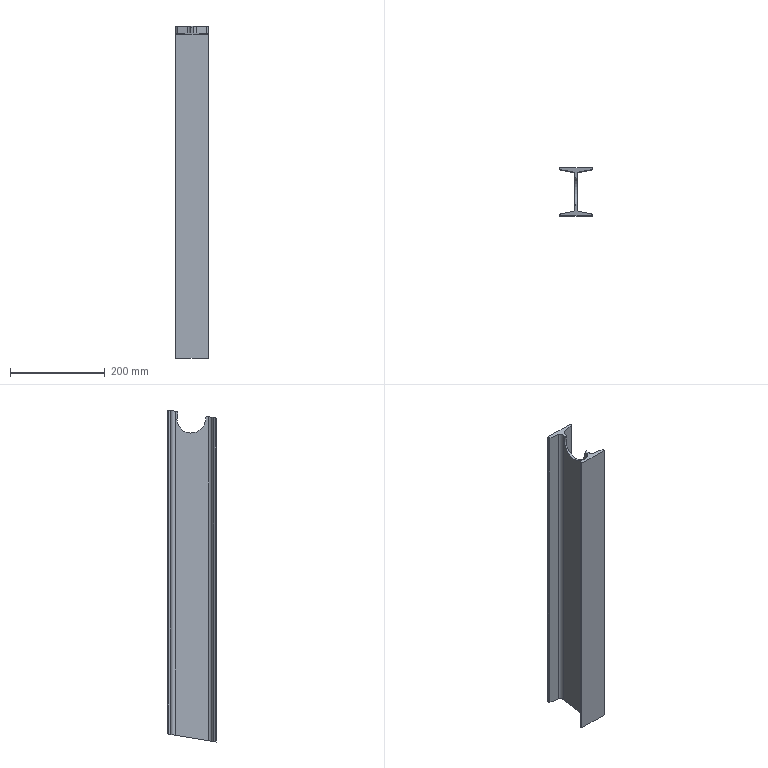Part | SolidWorks | features BaseBody 1 | 1 solid | 26 faces | box 67.6 x 101.6 x 699.36 mm | volume 938679 mm3 | plane 17 | cylinder 9 | commonest cylinder face diameters 5.6 x4 14.8 x4 60 x1
STEP:
#1=CARTESIAN_POINT('',(13.688,4.326,0.));
#2=VERTEX_POINT('',#1);
#3=CARTESIAN_POINT('',(81.288,4.326,0.));
#4=VERTEX_POINT('',#3);
#5=CARTESIAN_POINT('',(81.288,4.326,0.));
#6=DIRECTION('',(1.,0.,0.));
#7=VECTOR('',#6,1000.);
#8=LINE('',#5,#7);
#9=EDGE_CURVE('',#2,#4,#8,.T.);
#10=ORIENTED_EDGE('',*,*,#9,.T.);
#11=CARTESIAN_POINT('',(81.288,4.326,682.358));
#12=VERTEX_POINT('',#11);
#13=CARTESIAN_POINT('',(81.288,4.326,0.));
#14=DIRECTION('',(0.,0.,1.));
#15=VECTOR('',#14,1000.);
#16=LINE('',#13,#15);
#17=EDGE_CURVE('',#4,#12,#16,.T.);
#18=ORIENTED_EDGE('',*,*,#17,.T.);
#19=CARTESIAN_POINT('',(13.688,4.326,682.358));
#20=VERTEX_POINT('',#19);
#21=CARTESIAN_POINT('',(81.288,4.326,682.358));
#22=DIRECTION('',(-1.,0.,0.));
#23=VECTOR('',#22,1000.);
#24=LINE('',#21,#23);
#25=EDGE_CURVE('',#12,#20,#24,.T.);
#26=ORIENTED_EDGE('',*,*,#25,.T.);
#27=CARTESIAN_POINT('',(13.688,4.326,0.));
#28=DIRECTION('',(0.,0.,-1.));
#29=VECTOR('',#28,1000.);
#30=LINE('',#27,#29);
#31=EDGE_CURVE('',#20,#2,#30,.T.);
#32=ORIENTED_EDGE('',*,*,#31,.T.);
#33=EDGE_LOOP('',(#10,#18,#26,#32));
#34=FACE_OUTER_BOUND('',#33,.T.);
#35=CARTESIAN_POINT('',(81.288,4.326,0.));
#36=DIRECTION('',(0.,-1.,0.));
#37=DIRECTION('',(0.,0.,-1.));
#38=AXIS2_PLACEMENT_3D('',#35,#36,#37);
#39=PLANE('',#38);
#40=ADVANCED_FACE('',(#34),#39,.T.);
#41=CARTESIAN_POINT('',(81.288,6.296,0.3297));
#42=VERTEX_POINT('',#41);
#43=CARTESIAN_POINT('',(81.288,4.326,0.));
#44=DIRECTION('',(0.,0.9863,0.165));
#45=VECTOR('',#44,1000.);
#46=LINE('',#43,#45);
#47=EDGE_CURVE('',#4,#42,#46,.T.);
#48=ORIENTED_EDGE('',*,*,#47,.T.);
#49=CARTESIAN_POINT('',(81.288,6.296,682.688));
#50=VERTEX_POINT('',#49);
#51=CARTESIAN_POINT('',(81.288,6.296,0.));
#52=DIRECTION('',(0.,0.,1.));
#53=VECTOR('',#52,1000.);
#54=LINE('',#51,#53);
#55=EDGE_CURVE('',#42,#50,#54,.T.);
#56=ORIENTED_EDGE('',*,*,#55,.T.);
#57=CARTESIAN_POINT('',(81.288,6.296,682.688));
#58=DIRECTION('',(0.,-0.9863,-0.165));
#59=VECTOR('',#58,1000.);
#60=LINE('',#57,#59);
#61=EDGE_CURVE('',#50,#12,#60,.T.);
#62=ORIENTED_EDGE('',*,*,#61,.T.);
#63=ORIENTED_EDGE('',*,*,#17,.F.);
#64=EDGE_LOOP('',(#48,#56,#62,#63));
#65=FACE_OUTER_BOUND('',#64,.T.);
#66=CARTESIAN_POINT('',(81.288,6.296,0.));
#67=DIRECTION('',(1.,0.,0.));
#68=DIRECTION('',(0.,1.,0.));
#69=AXIS2_PLACEMENT_3D('',#66,#67,#68);
#70=PLANE('',#69);
#71=ADVANCED_FACE('',(#65),#70,.T.);
#72=CARTESIAN_POINT('',(81.288,105.926,17.002));
#73=VERTEX_POINT('',#72);
#74=CARTESIAN_POINT('',(13.688,105.926,17.002));
#75=VERTEX_POINT('',#74);
#76=CARTESIAN_POINT('',(47.488,105.926,17.002));
#77=DIRECTION('',(-1.,0.,0.));
#78=VECTOR('',#77,1000.);
#79=LINE('',#76,#78);
#80=EDGE_CURVE('',#73,#75,#79,.T.);
#81=ORIENTED_EDGE('',*,*,#80,.F.);
#82=CARTESIAN_POINT('',(81.288,103.955,16.672));
#83=VERTEX_POINT('',#82);
#84=CARTESIAN_POINT('',(81.288,54.429,8.384));
#85=DIRECTION('',(0.,0.9863,0.165));
#86=VECTOR('',#85,1000.);
#87=LINE('',#84,#86);
#88=EDGE_CURVE('',#83,#73,#87,.T.);
#89=ORIENTED_EDGE('',*,*,#88,.F.);
#90=CARTESIAN_POINT('',(78.95,101.193,16.21));
#91=VERTEX_POINT('',#90);
#92=CARTESIAN_POINT('',(78.95,101.193,16.21));
#93=CARTESIAN_POINT('',(80.362,101.43,16.25));
#94=CARTESIAN_POINT('',(81.288,102.523,16.433));
#95=CARTESIAN_POINT('',(81.288,103.955,16.672));
#96=(BOUNDED_CURVE()B_SPLINE_CURVE(3,(#92,#93,#94,#95),.UNSPECIFIED.,.F.,.F.)B_SPLINE_CURVE_WITH_KNOTS((4,4),(3.307,4.712),.UNSPECIFIED.)CURVE()GEOMETRIC_REPRESENTATION_ITEM()RATIONAL_B_SPLINE_CURVE((1.,0.8422,0.8422,1.))REPRESENTATION_ITEM(''));
#97=EDGE_CURVE('',#91,#83,#96,.T.);
#98=ORIENTED_EDGE('',*,*,#97,.F.);
#99=CARTESIAN_POINT('',(56.066,97.364,15.569));
#100=VERTEX_POINT('',#99);
#101=CARTESIAN_POINT('',(56.066,97.364,15.569));
#102=DIRECTION('',(0.9859,0.165,0.02761));
#103=VECTOR('',#102,1000.);
#104=LINE('',#101,#103);
#105=EDGE_CURVE('',#100,#91,#104,.T.);
#106=ORIENTED_EDGE('',*,*,#105,.F.);
#107=CARTESIAN_POINT('',(49.888,90.066,14.348));
#108=VERTEX_POINT('',#107);
#109=CARTESIAN_POINT('',(49.888,90.066,14.348));
#110=CARTESIAN_POINT('',(49.888,93.851,14.981));
#111=CARTESIAN_POINT('',(52.333,96.739,15.465));
#112=CARTESIAN_POINT('',(56.066,97.364,15.569));
#113=(BOUNDED_CURVE()B_SPLINE_CURVE(3,(#109,#110,#111,#112),.UNSPECIFIED.,.F.,.T.)B_SPLINE_CURVE_WITH_KNOTS((4,4),(4.712,6.117),.UNSPECIFIED.)CURVE()GEOMETRIC_REPRESENTATION_ITEM()RATIONAL_B_SPLINE_CURVE((1.,0.8422,0.8422,1.))REPRESENTATION_ITEM(''));
#114=EDGE_CURVE('',#108,#100,#113,.T.);
#115=ORIENTED_EDGE('',*,*,#114,.F.);
#116=CARTESIAN_POINT('',(49.888,20.186,2.654));
#117=VERTEX_POINT('',#116);
#118=CARTESIAN_POINT('',(49.888,54.429,8.384));
#119=DIRECTION('',(0.,0.9863,0.165));
#120=VECTOR('',#119,1000.);
#121=LINE('',#118,#120);
#122=EDGE_CURVE('',#117,#108,#121,.T.);
#123=ORIENTED_EDGE('',*,*,#122,.F.);
#124=CARTESIAN_POINT('',(56.066,12.887,1.433));
#125=VERTEX_POINT('',#124);
#126=CARTESIAN_POINT('',(56.066,12.887,1.433));
#127=CARTESIAN_POINT('',(52.333,13.512,1.537));
#128=CARTESIAN_POINT('',(49.888,16.401,2.021));
#129=CARTESIAN_POINT('',(49.888,20.186,2.654));
#130=(BOUNDED_CURVE()B_SPLINE_CURVE(3,(#126,#127,#128,#129),.UNSPECIFIED.,.F.,.F.)B_SPLINE_CURVE_WITH_KNOTS((4,4),(3.307,4.712),.UNSPECIFIED.)CURVE()GEOMETRIC_REPRESENTATION_ITEM()RATIONAL_B_SPLINE_CURVE((1.,0.8422,0.8422,1.))REPRESENTATION_ITEM(''));
#131=EDGE_CURVE('',#125,#117,#130,.T.);
#132=ORIENTED_EDGE('',*,*,#131,.F.);
#133=CARTESIAN_POINT('',(78.95,9.058,0.7919));
#134=VERTEX_POINT('',#133);
#135=CARTESIAN_POINT('',(78.95,9.058,0.7919));
#136=DIRECTION('',(-0.9859,0.165,0.02761));
#137=VECTOR('',#136,1000.);
#138=LINE('',#135,#137);
#139=EDGE_CURVE('',#134,#125,#138,.T.);
#140=ORIENTED_EDGE('',*,*,#139,.F.);
#141=CARTESIAN_POINT('',(81.288,6.296,0.3297));
#142=CARTESIAN_POINT('',(81.288,7.728,0.5694));
#143=CARTESIAN_POINT('',(80.362,8.821,0.7523));
#144=CARTESIAN_POINT('',(78.95,9.058,0.7919));
#145=(BOUNDED_CURVE()B_SPLINE_CURVE(3,(#141,#142,#143,#144),.UNSPECIFIED.,.F.,.F.)B_SPLINE_CURVE_WITH_KNOTS((4,4),(4.712,6.117),.UNSPECIFIED.)CURVE()GEOMETRIC_REPRESENTATION_ITEM()RATIONAL_B_SPLINE_CURVE((1.,0.8422,0.8422,1.))REPRESENTATION_ITEM(''));
#146=EDGE_CURVE('',#42,#134,#145,.T.);
#147=ORIENTED_EDGE('',*,*,#146,.F.);
#148=ORIENTED_EDGE('',*,*,#47,.F.);
#149=ORIENTED_EDGE('',*,*,#9,.F.);
#150=CARTESIAN_POINT('',(13.688,6.296,0.3297));
#151=VERTEX_POINT('',#150);
#152=CARTESIAN_POINT('',(13.688,54.429,8.384));
#153=DIRECTION('',(0.,-0.9863,-0.165));
#154=VECTOR('',#153,1000.);
#155=LINE('',#152,#154);
#156=EDGE_CURVE('',#151,#2,#155,.T.);
#157=ORIENTED_EDGE('',*,*,#156,.F.);
#158=CARTESIAN_POINT('',(16.026,9.058,0.7919));
#159=VERTEX_POINT('',#158);
#160=CARTESIAN_POINT('',(16.026,9.058,0.7919));
#161=CARTESIAN_POINT('',(14.613,8.821,0.7523));
#162=CARTESIAN_POINT('',(13.688,7.728,0.5694));
#163=CARTESIAN_POINT('',(13.688,6.296,0.3297));
#164=(BOUNDED_CURVE()B_SPLINE_CURVE(3,(#160,#161,#162,#163),.UNSPECIFIED.,.F.,.T.)B_SPLINE_CURVE_WITH_KNOTS((4,4),(0.1658,1.571),.UNSPECIFIED.)CURVE()GEOMETRIC_REPRESENTATION_ITEM()RATIONAL_B_SPLINE_CURVE((1.,0.8422,0.8422,1.))REPRESENTATION_ITEM(''));
#165=EDGE_CURVE('',#159,#151,#164,.T.);
#166=ORIENTED_EDGE('',*,*,#165,.F.);
#167=CARTESIAN_POINT('',(38.909,12.887,1.433));
#168=VERTEX_POINT('',#167);
#169=CARTESIAN_POINT('',(38.909,12.887,1.433));
#170=DIRECTION('',(-0.9859,-0.165,-0.02761));
#171=VECTOR('',#170,1000.);
#172=LINE('',#169,#171);
#173=EDGE_CURVE('',#168,#159,#172,.T.);
#174=ORIENTED_EDGE('',*,*,#173,.F.);
#175=CARTESIAN_POINT('',(45.088,20.186,2.654));
#176=VERTEX_POINT('',#175);
#177=CARTESIAN_POINT('',(45.088,20.186,2.654));
#178=CARTESIAN_POINT('',(45.088,16.401,2.021));
#179=CARTESIAN_POINT('',(42.642,13.512,1.537));
#180=CARTESIAN_POINT('',(38.909,12.887,1.433));
#181=(BOUNDED_CURVE()B_SPLINE_CURVE(3,(#177,#178,#179,#180),.UNSPECIFIED.,.F.,.F.)B_SPLINE_CURVE_WITH_KNOTS((4,4),(1.571,2.976),.UNSPECIFIED.)CURVE()GEOMETRIC_REPRESENTATION_ITEM()RATIONAL_B_SPLINE_CURVE((1.,0.8422,0.8422,1.))REPRESENTATION_ITEM(''));
#182=EDGE_CURVE('',#176,#168,#181,.T.);
#183=ORIENTED_EDGE('',*,*,#182,.F.);
#184=CARTESIAN_POINT('',(45.088,90.066,14.348));
#185=VERTEX_POINT('',#184);
#186=CARTESIAN_POINT('',(45.088,54.429,8.384));
#187=DIRECTION('',(0.,-0.9863,-0.165));
#188=VECTOR('',#187,1000.);
#189=LINE('',#186,#188);
#190=EDGE_CURVE('',#185,#176,#189,.T.);
#191=ORIENTED_EDGE('',*,*,#190,.F.);
#192=CARTESIAN_POINT('',(38.909,97.364,15.569));
#193=VERTEX_POINT('',#192);
#194=CARTESIAN_POINT('',(38.909,97.364,15.569));
#195=CARTESIAN_POINT('',(42.642,96.739,15.465));
#196=CARTESIAN_POINT('',(45.088,93.851,14.981));
#197=CARTESIAN_POINT('',(45.088,90.066,14.348));
#198=(BOUNDED_CURVE()B_SPLINE_CURVE(3,(#194,#195,#196,#197),.UNSPECIFIED.,.F.,.F.)B_SPLINE_CURVE_WITH_KNOTS((4,4),(0.1658,1.571),.UNSPECIFIED.)CURVE()GEOMETRIC_REPRESENTATION_ITEM()RATIONAL_B_SPLINE_CURVE((1.,0.8422,0.8422,1.))REPRESENTATION_ITEM(''));
#199=EDGE_CURVE('',#193,#185,#198,.T.);
#200=ORIENTED_EDGE('',*,*,#199,.F.);
#201=CARTESIAN_POINT('',(16.026,101.193,16.21));
#202=VERTEX_POINT('',#201);
#203=CARTESIAN_POINT('',(16.026,101.193,16.21));
#204=DIRECTION('',(0.9859,-0.165,-0.02761));
#205=VECTOR('',#204,1000.);
#206=LINE('',#203,#205);
#207=EDGE_CURVE('',#202,#193,#206,.T.);
#208=ORIENTED_EDGE('',*,*,#207,.F.);
#209=CARTESIAN_POINT('',(13.688,103.955,16.672));
#210=VERTEX_POINT('',#209);
#211=CARTESIAN_POINT('',(13.688,103.955,16.672));
#212=CARTESIAN_POINT('',(13.688,102.523,16.433));
#213=CARTESIAN_POINT('',(14.613,101.43,16.25));
#214=CARTESIAN_POINT('',(16.026,101.193,16.21));
#215=(BOUNDED_CURVE()B_SPLINE_CURVE(3,(#211,#212,#213,#214),.UNSPECIFIED.,.F.,.F.)B_SPLINE_CURVE_WITH_KNOTS((4,4),(1.571,2.976),.UNSPECIFIED.)CURVE()GEOMETRIC_REPRESENTATION_ITEM()RATIONAL_B_SPLINE_CURVE((1.,0.8422,0.8422,1.))REPRESENTATION_ITEM(''));
#216=EDGE_CURVE('',#210,#202,#215,.T.);
#217=ORIENTED_EDGE('',*,*,#216,.F.);
#218=CARTESIAN_POINT('',(13.688,54.429,8.384));
#219=DIRECTION('',(0.,-0.9863,-0.165));
#220=VECTOR('',#219,1000.);
#221=LINE('',#218,#220);
#222=EDGE_CURVE('',#75,#210,#221,.T.);
#223=ORIENTED_EDGE('',*,*,#222,.F.);
#224=EDGE_LOOP('',(#81,#89,#98,#106,#115,#123,#132,#140,#147,#148,#149,#157,#166,#174,#183,#191,#200,#208,#217,#223));
#225=FACE_OUTER_BOUND('',#224,.T.);
#226=CARTESIAN_POINT('',(47.488,54.429,8.384));
#227=DIRECTION('',(0.,-0.165,0.9863));
#228=DIRECTION('',(0.,-0.9863,-0.165));
#229=AXIS2_PLACEMENT_3D('',#226,#227,#228);
#230=PLANE('',#229);
#231=ADVANCED_FACE('',(#225),#230,.F.);
#232=ORIENTED_EDGE('',*,*,#156,.T.);
#233=ORIENTED_EDGE('',*,*,#31,.F.);
#234=CARTESIAN_POINT('',(13.688,6.296,682.688));
#235=VERTEX_POINT('',#234);
#236=CARTESIAN_POINT('',(13.688,4.326,682.358));
#237=DIRECTION('',(0.,0.9863,0.165));
#238=VECTOR('',#237,1000.);
#239=LINE('',#236,#238);
#240=EDGE_CURVE('',#20,#235,#239,.T.);
#241=ORIENTED_EDGE('',*,*,#240,.T.);
#242=CARTESIAN_POINT('',(13.688,6.296,0.));
#243=DIRECTION('',(0.,0.,-1.));
#244=VECTOR('',#243,1000.);
#245=LINE('',#242,#244);
#246=EDGE_CURVE('',#235,#151,#245,.T.);
#247=ORIENTED_EDGE('',*,*,#246,.T.);
#248=EDGE_LOOP('',(#232,#233,#241,#247));
#249=FACE_OUTER_BOUND('',#248,.T.);
#250=CARTESIAN_POINT('',(13.688,4.326,0.));
#251=DIRECTION('',(-1.,0.,0.));
#252=DIRECTION('',(0.,-1.,0.));
#253=AXIS2_PLACEMENT_3D('',#250,#251,#252);
#254=PLANE('',#253);
#255=ADVANCED_FACE('',(#249),#254,.T.);
#256=CARTESIAN_POINT('',(56.066,12.887,683.791));
#257=VERTEX_POINT('',#256);
#258=CARTESIAN_POINT('',(49.888,20.186,685.012));
#259=VERTEX_POINT('',#258);
#260=CARTESIAN_POINT('',(56.066,12.887,683.791));
#261=CARTESIAN_POINT('',(52.333,13.512,683.895));
#262=CARTESIAN_POINT('',(49.888,16.401,684.379));
#263=CARTESIAN_POINT('',(49.888,20.186,685.012));
#264=(BOUNDED_CURVE()B_SPLINE_CURVE(3,(#260,#261,#262,#263),.UNSPECIFIED.,.F.,.F.)B_SPLINE_CURVE_WITH_KNOTS((4,4),(3.307,4.712),.UNSPECIFIED.)CURVE()GEOMETRIC_REPRESENTATION_ITEM()RATIONAL_B_SPLINE_CURVE((1.,0.8422,0.8422,1.))REPRESENTATION_ITEM(''));
#265=EDGE_CURVE('',#257,#259,#264,.T.);
#266=ORIENTED_EDGE('',*,*,#265,.T.);
#267=CARTESIAN_POINT('',(49.888,25.536,685.907));
#268=VERTEX_POINT('',#267);
#269=CARTESIAN_POINT('',(49.888,55.822,690.976));
#270=DIRECTION('',(0.,0.9863,0.165));
#271=VECTOR('',#270,1000.);
#272=LINE('',#269,#271);
#273=EDGE_CURVE('',#259,#268,#272,.T.);
#274=ORIENTED_EDGE('',*,*,#273,.T.);
#275=CARTESIAN_POINT('',(45.088,25.536,685.907));
#276=VERTEX_POINT('',#275);
#277=CARTESIAN_POINT('',(47.488,25.536,685.907));
#278=DIRECTION('',(-1.,0.,0.));
#279=VECTOR('',#278,1000.);
#280=LINE('',#277,#279);
#281=EDGE_CURVE('',#268,#276,#280,.T.);
#282=ORIENTED_EDGE('',*,*,#281,.T.);
#283=CARTESIAN_POINT('',(45.088,20.186,685.012));
#284=VERTEX_POINT('',#283);
#285=CARTESIAN_POINT('',(45.088,55.822,690.976));
#286=DIRECTION('',(0.,-0.9863,-0.165));
#287=VECTOR('',#286,1000.);
#288=LINE('',#285,#287);
#289=EDGE_CURVE('',#276,#284,#288,.T.);
#290=ORIENTED_EDGE('',*,*,#289,.T.);
#291=CARTESIAN_POINT('',(38.909,12.887,683.791));
#292=VERTEX_POINT('',#291);
#293=CARTESIAN_POINT('',(45.088,20.186,685.012));
#294=CARTESIAN_POINT('',(45.088,16.401,684.379));
#295=CARTESIAN_POINT('',(42.642,13.512,683.895));
#296=CARTESIAN_POINT('',(38.909,12.887,683.791));
#297=(BOUNDED_CURVE()B_SPLINE_CURVE(3,(#293,#294,#295,#296),.UNSPECIFIED.,.F.,.T.)B_SPLINE_CURVE_WITH_KNOTS((4,4),(1.571,2.976),.UNSPECIFIED.)CURVE()GEOMETRIC_REPRESENTATION_ITEM()RATIONAL_B_SPLINE_CURVE((1.,0.8422,0.8422,1.))REPRESENTATION_ITEM(''));
#298=EDGE_CURVE('',#284,#292,#297,.T.);
#299=ORIENTED_EDGE('',*,*,#298,.T.);
#300=CARTESIAN_POINT('',(16.026,9.058,683.15));
#301=VERTEX_POINT('',#300);
#302=CARTESIAN_POINT('',(38.909,12.887,683.791));
#303=DIRECTION('',(-0.9859,-0.165,-0.02761));
#304=VECTOR('',#303,1000.);
#305=LINE('',#302,#304);
#306=EDGE_CURVE('',#292,#301,#305,.T.);
#307=ORIENTED_EDGE('',*,*,#306,.T.);
#308=CARTESIAN_POINT('',(16.026,9.058,683.15));
#309=CARTESIAN_POINT('',(14.613,8.821,683.11));
#310=CARTESIAN_POINT('',(13.688,7.728,682.927));
#311=CARTESIAN_POINT('',(13.688,6.296,682.688));
#312=(BOUNDED_CURVE()B_SPLINE_CURVE(3,(#308,#309,#310,#311),.UNSPECIFIED.,.F.,.F.)B_SPLINE_CURVE_WITH_KNOTS((4,4),(0.1658,1.571),.UNSPECIFIED.)CURVE()GEOMETRIC_REPRESENTATION_ITEM()RATIONAL_B_SPLINE_CURVE((1.,0.8422,0.8422,1.))REPRESENTATION_ITEM(''));
#313=EDGE_CURVE('',#301,#235,#312,.T.);
#314=ORIENTED_EDGE('',*,*,#313,.T.);
#315=ORIENTED_EDGE('',*,*,#240,.F.);
#316=ORIENTED_EDGE('',*,*,#25,.F.);
#317=ORIENTED_EDGE('',*,*,#61,.F.);
#318=CARTESIAN_POINT('',(78.95,9.058,683.15));
#319=VERTEX_POINT('',#318);
#320=CARTESIAN_POINT('',(81.288,6.296,682.688));
#321=CARTESIAN_POINT('',(81.288,7.728,682.927));
#322=CARTESIAN_POINT('',(80.362,8.821,683.11));
#323=CARTESIAN_POINT('',(78.95,9.058,683.15));
#324=(BOUNDED_CURVE()B_SPLINE_CURVE(3,(#320,#321,#322,#323),.UNSPECIFIED.,.F.,.F.)B_SPLINE_CURVE_WITH_KNOTS((4,4),(4.712,6.117),.UNSPECIFIED.)CURVE()GEOMETRIC_REPRESENTATION_ITEM()RATIONAL_B_SPLINE_CURVE((1.,0.8422,0.8422,1.))REPRESENTATION_ITEM(''));
#325=EDGE_CURVE('',#50,#319,#324,.T.);
#326=ORIENTED_EDGE('',*,*,#325,.T.);
#327=CARTESIAN_POINT('',(78.95,9.058,683.15));
#328=DIRECTION('',(-0.9859,0.165,0.02761));
#329=VECTOR('',#328,1000.);
#330=LINE('',#327,#329);
#331=EDGE_CURVE('',#319,#257,#330,.T.);
#332=ORIENTED_EDGE('',*,*,#331,.T.);
#333=EDGE_LOOP('',(#266,#274,#282,#290,#299,#307,#314,#315,#316,#317,#326,#332));
#334=FACE_OUTER_BOUND('',#333,.T.);
#335=CARTESIAN_POINT('',(47.488,55.822,690.976));
#336=DIRECTION('',(0.,-0.165,0.9863));
#337=DIRECTION('',(0.,-0.9863,-0.165));
#338=AXIS2_PLACEMENT_3D('',#335,#336,#337);
#339=PLANE('',#338);
#340=ADVANCED_FACE('',(#334),#339,.T.);
#341=ORIENTED_EDGE('',*,*,#146,.T.);
#342=CARTESIAN_POINT('',(78.95,9.058,0.));
#343=DIRECTION('',(0.,0.,1.));
#344=VECTOR('',#343,1000.);
#345=LINE('',#342,#344);
#346=EDGE_CURVE('',#134,#319,#345,.T.);
#347=ORIENTED_EDGE('',*,*,#346,.T.);
#348=ORIENTED_EDGE('',*,*,#325,.F.);
#349=ORIENTED_EDGE('',*,*,#55,.F.);
#350=EDGE_LOOP('',(#341,#347,#348,#349));
#351=FACE_OUTER_BOUND('',#350,.T.);
#352=CARTESIAN_POINT('',(78.488,6.296,0.));
#353=DIRECTION('',(0.,0.,1.));
#354=DIRECTION('',(1.,0.,0.));
#355=AXIS2_PLACEMENT_3D('',#352,#353,#354);
#356=CYLINDRICAL_SURFACE('',#355,2.8);
#357=ADVANCED_FACE('',(#351),#356,.T.);
#358=ORIENTED_EDGE('',*,*,#222,.T.);
#359=CARTESIAN_POINT('',(13.688,103.955,699.03));
#360=VERTEX_POINT('',#359);
#361=CARTESIAN_POINT('',(13.688,103.955,0.));
#362=DIRECTION('',(0.,0.,1.));
#363=VECTOR('',#362,1000.);
#364=LINE('',#361,#363);
#365=EDGE_CURVE('',#210,#360,#364,.T.);
#366=ORIENTED_EDGE('',*,*,#365,.T.);
#367=CARTESIAN_POINT('',(13.688,105.926,699.36));
#368=VERTEX_POINT('',#367);
#369=CARTESIAN_POINT('',(13.688,103.955,699.03));
#370=DIRECTION('',(0.,0.9863,0.165));
#371=VECTOR('',#370,1000.);
#372=LINE('',#369,#371);
#373=EDGE_CURVE('',#360,#368,#372,.T.);
#374=ORIENTED_EDGE('',*,*,#373,.T.);
#375=CARTESIAN_POINT('',(13.688,105.926,0.));
#376=DIRECTION('',(0.,0.,-1.));
#377=VECTOR('',#376,1000.);
#378=LINE('',#375,#377);
#379=EDGE_CURVE('',#368,#75,#378,.T.);
#380=ORIENTED_EDGE('',*,*,#379,.T.);
#381=EDGE_LOOP('',(#358,#366,#374,#380));
#382=FACE_OUTER_BOUND('',#381,.T.);
#383=CARTESIAN_POINT('',(13.688,103.955,0.));
#384=DIRECTION('',(-1.,0.,0.));
#385=DIRECTION('',(0.,0.,1.));
#386=AXIS2_PLACEMENT_3D('',#383,#384,#385);
#387=PLANE('',#386);
#388=ADVANCED_FACE('',(#382),#387,.T.);
#389=ORIENTED_EDGE('',*,*,#80,.T.);
#390=ORIENTED_EDGE('',*,*,#379,.F.);
#391=CARTESIAN_POINT('',(81.288,105.926,699.36));
#392=VERTEX_POINT('',#391);
#393=CARTESIAN_POINT('',(13.688,105.926,699.36));
#394=DIRECTION('',(1.,0.,0.));
#395=VECTOR('',#394,1000.);
#396=LINE('',#393,#395);
#397=EDGE_CURVE('',#368,#392,#396,.T.);
#398=ORIENTED_EDGE('',*,*,#397,.T.);
#399=CARTESIAN_POINT('',(81.288,105.926,0.));
#400=DIRECTION('',(0.,0.,-1.));
#401=VECTOR('',#400,1000.);
#402=LINE('',#399,#401);
#403=EDGE_CURVE('',#392,#73,#402,.T.);
#404=ORIENTED_EDGE('',*,*,#403,.T.);
#405=EDGE_LOOP('',(#389,#390,#398,#404));
#406=FACE_OUTER_BOUND('',#405,.T.);
#407=CARTESIAN_POINT('',(13.688,105.926,0.));
#408=DIRECTION('',(0.,1.,0.));
#409=DIRECTION('',(0.,0.,1.));
#410=AXIS2_PLACEMENT_3D('',#407,#408,#409);
#411=PLANE('',#410);
#412=ADVANCED_FACE('',(#406),#411,.T.);
#413=ORIENTED_EDGE('',*,*,#88,.T.);
#414=ORIENTED_EDGE('',*,*,#403,.F.);
#415=CARTESIAN_POINT('',(81.288,103.955,699.03));
#416=VERTEX_POINT('',#415);
#417=CARTESIAN_POINT('',(81.288,105.926,699.36));
#418=DIRECTION('',(0.,-0.9863,-0.165));
#419=VECTOR('',#418,1000.);
#420=LINE('',#417,#419);
#421=EDGE_CURVE('',#392,#416,#420,.T.);
#422=ORIENTED_EDGE('',*,*,#421,.T.);
#423=CARTESIAN_POINT('',(81.288,103.955,0.));
#424=DIRECTION('',(0.,0.,-1.));
#425=VECTOR('',#424,1000.);
#426=LINE('',#423,#425);
#427=EDGE_CURVE('',#416,#83,#426,.T.);
#428=ORIENTED_EDGE('',*,*,#427,.T.);
#429=EDGE_LOOP('',(#413,#414,#422,#428));
#430=FACE_OUTER_BOUND('',#429,.T.);
#431=CARTESIAN_POINT('',(81.288,105.926,0.));
#432=DIRECTION('',(1.,0.,0.));
#433=DIRECTION('',(0.,1.,0.));
#434=AXIS2_PLACEMENT_3D('',#431,#432,#433);
#435=PLANE('',#434);
#436=ADVANCED_FACE('',(#430),#435,.T.);
#437=ORIENTED_EDGE('',*,*,#97,.T.);
#438=ORIENTED_EDGE('',*,*,#427,.F.);
#439=CARTESIAN_POINT('',(78.95,101.193,698.568));
#440=VERTEX_POINT('',#439);
#441=CARTESIAN_POINT('',(81.288,103.955,699.03));
#442=CARTESIAN_POINT('',(81.288,102.523,698.791));
#443=CARTESIAN_POINT('',(80.362,101.43,698.608));
#444=CARTESIAN_POINT('',(78.95,101.193,698.568));
#445=(BOUNDED_CURVE()B_SPLINE_CURVE(3,(#441,#442,#443,#444),.UNSPECIFIED.,.F.,.F.)B_SPLINE_CURVE_WITH_KNOTS((4,4),(1.571,2.976),.UNSPECIFIED.)CURVE()GEOMETRIC_REPRESENTATION_ITEM()RATIONAL_B_SPLINE_CURVE((1.,0.8422,0.8422,1.))REPRESENTATION_ITEM(''));
#446=EDGE_CURVE('',#416,#440,#445,.T.);
#447=ORIENTED_EDGE('',*,*,#446,.T.);
#448=CARTESIAN_POINT('',(78.95,101.193,0.));
#449=DIRECTION('',(0.,0.,-1.));
#450=VECTOR('',#449,1000.);
#451=LINE('',#448,#450);
#452=EDGE_CURVE('',#440,#91,#451,.T.);
#453=ORIENTED_EDGE('',*,*,#452,.T.);
#454=EDGE_LOOP('',(#437,#438,#447,#453));
#455=FACE_OUTER_BOUND('',#454,.T.);
#456=CARTESIAN_POINT('',(78.488,103.955,0.));
#457=DIRECTION('',(0.,0.,1.));
#458=DIRECTION('',(1.,0.,0.));
#459=AXIS2_PLACEMENT_3D('',#456,#457,#458);
#460=CYLINDRICAL_SURFACE('',#459,2.8);
#461=ADVANCED_FACE('',(#455),#460,.T.);
#462=ORIENTED_EDGE('',*,*,#105,.T.);
#463=ORIENTED_EDGE('',*,*,#452,.F.);
#464=CARTESIAN_POINT('',(56.066,97.364,697.927));
#465=VERTEX_POINT('',#464);
#466=CARTESIAN_POINT('',(78.95,101.193,698.568));
#467=DIRECTION('',(-0.9859,-0.165,-0.02761));
#468=VECTOR('',#467,1000.);
#469=LINE('',#466,#468);
#470=EDGE_CURVE('',#440,#465,#469,.T.);
#471=ORIENTED_EDGE('',*,*,#470,.T.);
#472=CARTESIAN_POINT('',(56.066,97.364,0.));
#473=DIRECTION('',(0.,0.,-1.));
#474=VECTOR('',#473,1000.);
#475=LINE('',#472,#474);
#476=EDGE_CURVE('',#465,#100,#475,.T.);
#477=ORIENTED_EDGE('',*,*,#476,.T.);
#478=EDGE_LOOP('',(#462,#463,#471,#477));
#479=FACE_OUTER_BOUND('',#478,.T.);
#480=CARTESIAN_POINT('',(78.95,101.193,0.));
#481=DIRECTION('',(0.165,-0.9863,0.));
#482=DIRECTION('',(0.9863,0.165,0.));
#483=AXIS2_PLACEMENT_3D('',#480,#481,#482);
#484=PLANE('',#483);
#485=ADVANCED_FACE('',(#479),#484,.T.);
#486=CARTESIAN_POINT('',(49.888,90.066,696.706));
#487=VERTEX_POINT('',#486);
#488=CARTESIAN_POINT('',(49.888,90.066,0.));
#489=DIRECTION('',(0.,0.,1.));
#490=VECTOR('',#489,1000.);
#491=LINE('',#488,#490);
#492=EDGE_CURVE('',#108,#487,#491,.T.);
#493=ORIENTED_EDGE('',*,*,#492,.F.);
#494=ORIENTED_EDGE('',*,*,#114,.T.);
#495=ORIENTED_EDGE('',*,*,#476,.F.);
#496=CARTESIAN_POINT('',(49.888,90.066,696.706));
#497=CARTESIAN_POINT('',(49.888,93.851,697.339));
#498=CARTESIAN_POINT('',(52.333,96.739,697.823));
#499=CARTESIAN_POINT('',(56.066,97.364,697.927));
#500=(BOUNDED_CURVE()B_SPLINE_CURVE(3,(#496,#497,#498,#499),.UNSPECIFIED.,.F.,.F.)B_SPLINE_CURVE_WITH_KNOTS((4,4),(4.712,6.117),.UNSPECIFIED.)CURVE()GEOMETRIC_REPRESENTATION_ITEM()RATIONAL_B_SPLINE_CURVE((1.,0.8422,0.8422,1.))REPRESENTATION_ITEM(''));
#501=EDGE_CURVE('',#487,#465,#500,.T.);
#502=ORIENTED_EDGE('',*,*,#501,.F.);
#503=EDGE_LOOP('',(#493,#494,#495,#502));
#504=FACE_OUTER_BOUND('',#503,.T.);
#505=CARTESIAN_POINT('',(57.288,90.066,0.));
#506=DIRECTION('',(0.,0.,1.));
#507=DIRECTION('',(1.,0.,0.));
#508=AXIS2_PLACEMENT_3D('',#505,#506,#507);
#509=CYLINDRICAL_SURFACE('',#508,7.4);
#510=ADVANCED_FACE('',(#504),#509,.F.);
#511=ORIENTED_EDGE('',*,*,#492,.T.);
#512=CARTESIAN_POINT('',(49.888,84.714,695.81));
#513=VERTEX_POINT('',#512);
#514=CARTESIAN_POINT('',(49.888,90.066,696.706));
#515=DIRECTION('',(0.,-0.9863,-0.165));
#516=VECTOR('',#515,1000.);
#517=LINE('',#514,#516);
#518=EDGE_CURVE('',#487,#513,#517,.T.);
#519=ORIENTED_EDGE('',*,*,#518,.T.);
#520=CARTESIAN_POINT('',(49.888,86.435,685.845));
#521=VERTEX_POINT('',#520);
#522=CARTESIAN_POINT('',(49.888,84.714,695.81));
#523=DIRECTION('',(0.,0.1702,-0.9854));
#524=VECTOR('',#523,1000.);
#525=LINE('',#522,#524);
#526=EDGE_CURVE('',#513,#521,#525,.T.);
#527=ORIENTED_EDGE('',*,*,#526,.T.);
#528=CARTESIAN_POINT('',(49.888,27.311,675.633));
#529=VERTEX_POINT('',#528);
#530=CARTESIAN_POINT('',(49.888,56.873,680.739));
#531=DIRECTION('',(-1.,0.,0.));
#532=DIRECTION('',(0.,0.,1.));
#533=AXIS2_PLACEMENT_3D('',#530,#531,#532);
#534=CIRCLE('',#533,30.);
#535=EDGE_CURVE('',#521,#529,#534,.T.);
#536=ORIENTED_EDGE('',*,*,#535,.T.);
#537=CARTESIAN_POINT('',(49.888,27.311,675.633));
#538=DIRECTION('',(0.,-0.1702,0.9854));
#539=VECTOR('',#538,1000.);
#540=LINE('',#537,#539);
#541=EDGE_CURVE('',#529,#268,#540,.T.);
#542=ORIENTED_EDGE('',*,*,#541,.T.);
#543=ORIENTED_EDGE('',*,*,#273,.F.);
#544=CARTESIAN_POINT('',(49.888,20.186,0.));
#545=DIRECTION('',(0.,0.,-1.));
#546=VECTOR('',#545,1000.);
#547=LINE('',#544,#546);
#548=EDGE_CURVE('',#259,#117,#547,.T.);
#549=ORIENTED_EDGE('',*,*,#548,.T.);
#550=ORIENTED_EDGE('',*,*,#122,.T.);
#551=EDGE_LOOP('',(#511,#519,#527,#536,#542,#543,#549,#550));
#552=FACE_OUTER_BOUND('',#551,.T.);
#553=CARTESIAN_POINT('',(49.888,90.066,0.));
#554=DIRECTION('',(1.,0.,0.));
#555=DIRECTION('',(0.,0.,-1.));
#556=AXIS2_PLACEMENT_3D('',#553,#554,#555);
#557=PLANE('',#556);
#558=ADVANCED_FACE('',(#552),#557,.T.);
#559=CARTESIAN_POINT('',(56.066,12.887,0.));
#560=DIRECTION('',(0.,0.,1.));
#561=VECTOR('',#560,1000.);
#562=LINE('',#559,#561);
#563=EDGE_CURVE('',#125,#257,#562,.T.);
#564=ORIENTED_EDGE('',*,*,#563,.F.);
#565=ORIENTED_EDGE('',*,*,#131,.T.);
#566=ORIENTED_EDGE('',*,*,#548,.F.);
#567=ORIENTED_EDGE('',*,*,#265,.F.);
#568=EDGE_LOOP('',(#564,#565,#566,#567));
#569=FACE_OUTER_BOUND('',#568,.T.);
#570=CARTESIAN_POINT('',(57.288,20.186,0.));
#571=DIRECTION('',(0.,0.,1.));
#572=DIRECTION('',(1.,0.,0.));
#573=AXIS2_PLACEMENT_3D('',#570,#571,#572);
#574=CYLINDRICAL_SURFACE('',#573,7.4);
#575=ADVANCED_FACE('',(#569),#574,.F.);
#576=ORIENTED_EDGE('',*,*,#139,.T.);
#577=ORIENTED_EDGE('',*,*,#563,.T.);
#578=ORIENTED_EDGE('',*,*,#331,.F.);
#579=ORIENTED_EDGE('',*,*,#346,.F.);
#580=EDGE_LOOP('',(#576,#577,#578,#579));
#581=FACE_OUTER_BOUND('',#580,.T.);
#582=CARTESIAN_POINT('',(56.066,12.887,0.));
#583=DIRECTION('',(0.165,0.9863,0.));
#584=DIRECTION('',(-0.9863,0.165,0.));
#585=AXIS2_PLACEMENT_3D('',#582,#583,#584);
#586=PLANE('',#585);
#587=ADVANCED_FACE('',(#581),#586,.T.);
#588=ORIENTED_EDGE('',*,*,#165,.T.);
#589=ORIENTED_EDGE('',*,*,#246,.F.);
#590=ORIENTED_EDGE('',*,*,#313,.F.);
#591=CARTESIAN_POINT('',(16.026,9.058,0.));
#592=DIRECTION('',(0.,0.,-1.));
#593=VECTOR('',#592,1000.);
#594=LINE('',#591,#593);
#595=EDGE_CURVE('',#301,#159,#594,.T.);
#596=ORIENTED_EDGE('',*,*,#595,.T.);
#597=EDGE_LOOP('',(#588,#589,#590,#596));
#598=FACE_OUTER_BOUND('',#597,.T.);
#599=CARTESIAN_POINT('',(16.488,6.296,0.));
#600=DIRECTION('',(0.,0.,1.));
#601=DIRECTION('',(1.,0.,0.));
#602=AXIS2_PLACEMENT_3D('',#599,#600,#601);
#603=CYLINDRICAL_SURFACE('',#602,2.8);
#604=ADVANCED_FACE('',(#598),#603,.T.);
#605=ORIENTED_EDGE('',*,*,#173,.T.);
#606=ORIENTED_EDGE('',*,*,#595,.F.);
#607=ORIENTED_EDGE('',*,*,#306,.F.);
#608=CARTESIAN_POINT('',(38.909,12.887,0.));
#609=DIRECTION('',(0.,0.,-1.));
#610=VECTOR('',#609,1000.);
#611=LINE('',#608,#610);
#612=EDGE_CURVE('',#292,#168,#611,.T.);
#613=ORIENTED_EDGE('',*,*,#612,.T.);
#614=EDGE_LOOP('',(#605,#606,#607,#613));
#615=FACE_OUTER_BOUND('',#614,.T.);
#616=CARTESIAN_POINT('',(16.026,9.058,0.));
#617=DIRECTION('',(-0.165,0.9863,0.));
#618=DIRECTION('',(-0.9863,-0.165,0.));
#619=AXIS2_PLACEMENT_3D('',#616,#617,#618);
#620=PLANE('',#619);
#621=ADVANCED_FACE('',(#615),#620,.T.);
#622=CARTESIAN_POINT('',(45.088,20.186,0.));
#623=DIRECTION('',(0.,0.,1.));
#624=VECTOR('',#623,1000.);
#625=LINE('',#622,#624);
#626=EDGE_CURVE('',#176,#284,#625,.T.);
#627=ORIENTED_EDGE('',*,*,#626,.F.);
#628=ORIENTED_EDGE('',*,*,#182,.T.);
#629=ORIENTED_EDGE('',*,*,#612,.F.);
#630=ORIENTED_EDGE('',*,*,#298,.F.);
#631=EDGE_LOOP('',(#627,#628,#629,#630));
#632=FACE_OUTER_BOUND('',#631,.T.);
#633=CARTESIAN_POINT('',(37.688,20.186,0.));
#634=DIRECTION('',(0.,0.,1.));
#635=DIRECTION('',(1.,0.,0.));
#636=AXIS2_PLACEMENT_3D('',#633,#634,#635);
#637=CYLINDRICAL_SURFACE('',#636,7.4);
#638=ADVANCED_FACE('',(#632),#637,.F.);
#639=CARTESIAN_POINT('',(45.088,27.311,675.633));
#640=VERTEX_POINT('',#639);
#641=CARTESIAN_POINT('',(45.088,25.536,685.907));
#642=DIRECTION('',(0.,0.1702,-0.9854));
#643=VECTOR('',#642,1000.);
#644=LINE('',#641,#643);
#645=EDGE_CURVE('',#276,#640,#644,.T.);
#646=ORIENTED_EDGE('',*,*,#645,.T.);
#647=CARTESIAN_POINT('',(45.088,86.435,685.845));
#648=VERTEX_POINT('',#647);
#649=CARTESIAN_POINT('',(45.088,56.873,680.739));
#650=DIRECTION('',(1.,0.,0.));
#651=DIRECTION('',(0.,0.,1.));
#652=AXIS2_PLACEMENT_3D('',#649,#650,#651);
#653=CIRCLE('',#652,30.);
#654=EDGE_CURVE('',#640,#648,#653,.T.);
#655=ORIENTED_EDGE('',*,*,#654,.T.);
#656=CARTESIAN_POINT('',(45.088,84.714,695.81));
#657=VERTEX_POINT('',#656);
#658=CARTESIAN_POINT('',(45.088,86.435,685.845));
#659=DIRECTION('',(0.,-0.1702,0.9854));
#660=VECTOR('',#659,1000.);
#661=LINE('',#658,#660);
#662=EDGE_CURVE('',#648,#657,#661,.T.);
#663=ORIENTED_EDGE('',*,*,#662,.T.);
#664=CARTESIAN_POINT('',(45.088,90.066,696.706));
#665=VERTEX_POINT('',#664);
#666=CARTESIAN_POINT('',(45.088,84.714,695.81));
#667=DIRECTION('',(0.,0.9863,0.165));
#668=VECTOR('',#667,1000.);
#669=LINE('',#666,#668);
#670=EDGE_CURVE('',#657,#665,#669,.T.);
#671=ORIENTED_EDGE('',*,*,#670,.T.);
#672=CARTESIAN_POINT('',(45.088,90.066,0.));
#673=DIRECTION('',(0.,0.,-1.));
#674=VECTOR('',#673,1000.);
#675=LINE('',#672,#674);
#676=EDGE_CURVE('',#665,#185,#675,.T.);
#677=ORIENTED_EDGE('',*,*,#676,.T.);
#678=ORIENTED_EDGE('',*,*,#190,.T.);
#679=ORIENTED_EDGE('',*,*,#626,.T.);
#680=ORIENTED_EDGE('',*,*,#289,.F.);
#681=EDGE_LOOP('',(#646,#655,#663,#671,#677,#678,#679,#680));
#682=FACE_OUTER_BOUND('',#681,.T.);
#683=CARTESIAN_POINT('',(45.088,20.186,0.));
#684=DIRECTION('',(-1.,0.,0.));
#685=DIRECTION('',(0.,0.,1.));
#686=AXIS2_PLACEMENT_3D('',#683,#684,#685);
#687=PLANE('',#686);
#688=ADVANCED_FACE('',(#682),#687,.T.);
#689=CARTESIAN_POINT('',(38.909,97.364,697.927));
#690=VERTEX_POINT('',#689);
#691=CARTESIAN_POINT('',(38.909,97.364,0.));
#692=DIRECTION('',(0.,0.,1.));
#693=VECTOR('',#692,1000.);
#694=LINE('',#691,#693);
#695=EDGE_CURVE('',#193,#690,#694,.T.);
#696=ORIENTED_EDGE('',*,*,#695,.F.);
#697=ORIENTED_EDGE('',*,*,#199,.T.);
#698=ORIENTED_EDGE('',*,*,#676,.F.);
#699=CARTESIAN_POINT('',(38.909,97.364,697.927));
#700=CARTESIAN_POINT('',(42.642,96.739,697.823));
#701=CARTESIAN_POINT('',(45.088,93.851,697.339));
#702=CARTESIAN_POINT('',(45.088,90.066,696.706));
#703=(BOUNDED_CURVE()B_SPLINE_CURVE(3,(#699,#700,#701,#702),.UNSPECIFIED.,.F.,.F.)B_SPLINE_CURVE_WITH_KNOTS((4,4),(0.1658,1.571),.UNSPECIFIED.)CURVE()GEOMETRIC_REPRESENTATION_ITEM()RATIONAL_B_SPLINE_CURVE((1.,0.8422,0.8422,1.))REPRESENTATION_ITEM(''));
#704=EDGE_CURVE('',#690,#665,#703,.T.);
#705=ORIENTED_EDGE('',*,*,#704,.F.);
#706=EDGE_LOOP('',(#696,#697,#698,#705));
#707=FACE_OUTER_BOUND('',#706,.T.);
#708=CARTESIAN_POINT('',(37.688,90.066,0.));
#709=DIRECTION('',(0.,0.,1.));
#710=DIRECTION('',(1.,0.,0.));
#711=AXIS2_PLACEMENT_3D('',#708,#709,#710);
#712=CYLINDRICAL_SURFACE('',#711,7.4);
#713=ADVANCED_FACE('',(#707),#712,.F.);
#714=ORIENTED_EDGE('',*,*,#207,.T.);
#715=ORIENTED_EDGE('',*,*,#695,.T.);
#716=CARTESIAN_POINT('',(16.026,101.193,698.568));
#717=VERTEX_POINT('',#716);
#718=CARTESIAN_POINT('',(38.909,97.364,697.927));
#719=DIRECTION('',(-0.9859,0.165,0.02761));
#720=VECTOR('',#719,1000.);
#721=LINE('',#718,#720);
#722=EDGE_CURVE('',#690,#717,#721,.T.);
#723=ORIENTED_EDGE('',*,*,#722,.T.);
#724=CARTESIAN_POINT('',(16.026,101.193,0.));
#725=DIRECTION('',(0.,0.,-1.));
#726=VECTOR('',#725,1000.);
#727=LINE('',#724,#726);
#728=EDGE_CURVE('',#717,#202,#727,.T.);
#729=ORIENTED_EDGE('',*,*,#728,.T.);
#730=EDGE_LOOP('',(#714,#715,#723,#729));
#731=FACE_OUTER_BOUND('',#730,.T.);
#732=CARTESIAN_POINT('',(38.909,97.364,0.));
#733=DIRECTION('',(-0.165,-0.9863,0.));
#734=DIRECTION('',(0.9863,-0.165,0.));
#735=AXIS2_PLACEMENT_3D('',#732,#733,#734);
#736=PLANE('',#735);
#737=ADVANCED_FACE('',(#731),#736,.T.);
#738=ORIENTED_EDGE('',*,*,#216,.T.);
#739=ORIENTED_EDGE('',*,*,#728,.F.);
#740=CARTESIAN_POINT('',(16.026,101.193,698.568));
#741=CARTESIAN_POINT('',(14.613,101.43,698.608));
#742=CARTESIAN_POINT('',(13.688,102.523,698.791));
#743=CARTESIAN_POINT('',(13.688,103.955,699.03));
#744=(BOUNDED_CURVE()B_SPLINE_CURVE(3,(#740,#741,#742,#743),.UNSPECIFIED.,.F.,.T.)B_SPLINE_CURVE_WITH_KNOTS((4,4),(3.307,4.712),.UNSPECIFIED.)CURVE()GEOMETRIC_REPRESENTATION_ITEM()RATIONAL_B_SPLINE_CURVE((1.,0.8422,0.8422,1.))REPRESENTATION_ITEM(''));
#745=EDGE_CURVE('',#717,#360,#744,.T.);
#746=ORIENTED_EDGE('',*,*,#745,.T.);
#747=ORIENTED_EDGE('',*,*,#365,.F.);
#748=EDGE_LOOP('',(#738,#739,#746,#747));
#749=FACE_OUTER_BOUND('',#748,.T.);
#750=CARTESIAN_POINT('',(16.488,103.955,0.));
#751=DIRECTION('',(0.,0.,1.));
#752=DIRECTION('',(1.,0.,0.));
#753=AXIS2_PLACEMENT_3D('',#750,#751,#752);
#754=CYLINDRICAL_SURFACE('',#753,2.8);
#755=ADVANCED_FACE('',(#749),#754,.T.);
#756=ORIENTED_EDGE('',*,*,#541,.F.);
#757=CARTESIAN_POINT('',(49.888,27.311,675.633));
#758=DIRECTION('',(1.,0.,0.));
#759=VECTOR('',#758,1000.);
#760=LINE('',#757,#759);
#761=EDGE_CURVE('',#640,#529,#760,.T.);
#762=ORIENTED_EDGE('',*,*,#761,.F.);
#763=ORIENTED_EDGE('',*,*,#645,.F.);
#764=ORIENTED_EDGE('',*,*,#281,.F.);
#765=EDGE_LOOP('',(#756,#762,#763,#764));
#766=FACE_OUTER_BOUND('',#765,.T.);
#767=CARTESIAN_POINT('',(49.888,24.029,694.631));
#768=DIRECTION('',(0.,-0.9854,-0.1702));
#769=DIRECTION('',(0.,0.1702,-0.9854));
#770=AXIS2_PLACEMENT_3D('',#767,#768,#769);
#771=PLANE('',#770);
#772=ADVANCED_FACE('',(#766),#771,.F.);
#773=ORIENTED_EDGE('',*,*,#704,.T.);
#774=ORIENTED_EDGE('',*,*,#670,.F.);
#775=CARTESIAN_POINT('',(47.488,84.714,695.81));
#776=DIRECTION('',(1.,0.,0.));
#777=VECTOR('',#776,1000.);
#778=LINE('',#775,#777);
#779=EDGE_CURVE('',#657,#513,#778,.T.);
#780=ORIENTED_EDGE('',*,*,#779,.T.);
#781=ORIENTED_EDGE('',*,*,#518,.F.);
#782=ORIENTED_EDGE('',*,*,#501,.T.);
#783=ORIENTED_EDGE('',*,*,#470,.F.);
#784=ORIENTED_EDGE('',*,*,#446,.F.);
#785=ORIENTED_EDGE('',*,*,#421,.F.);
#786=ORIENTED_EDGE('',*,*,#397,.F.);
#787=ORIENTED_EDGE('',*,*,#373,.F.);
#788=ORIENTED_EDGE('',*,*,#745,.F.);
#789=ORIENTED_EDGE('',*,*,#722,.F.);
#790=EDGE_LOOP('',(#773,#774,#780,#781,#782,#783,#784,#785,#786,#787,#788,#789));
#791=FACE_OUTER_BOUND('',#790,.T.);
#792=CARTESIAN_POINT('',(47.488,55.822,690.976));
#793=DIRECTION('',(0.,-0.165,0.9863));
#794=DIRECTION('',(0.,-0.9863,-0.165));
#795=AXIS2_PLACEMENT_3D('',#792,#793,#794);
#796=PLANE('',#795);
#797=ADVANCED_FACE('',(#791),#796,.T.);
#798=ORIENTED_EDGE('',*,*,#761,.T.);
#799=ORIENTED_EDGE('',*,*,#535,.F.);
#800=CARTESIAN_POINT('',(49.888,86.435,685.845));
#801=DIRECTION('',(1.,0.,0.));
#802=VECTOR('',#801,1000.);
#803=LINE('',#800,#802);
#804=EDGE_CURVE('',#648,#521,#803,.T.);
#805=ORIENTED_EDGE('',*,*,#804,.F.);
#806=ORIENTED_EDGE('',*,*,#654,.F.);
#807=EDGE_LOOP('',(#798,#799,#805,#806));
#808=FACE_OUTER_BOUND('',#807,.T.);
#809=CARTESIAN_POINT('',(49.888,56.873,680.739));
#810=DIRECTION('',(-1.,0.,0.));
#811=DIRECTION('',(0.,0.,1.));
#812=AXIS2_PLACEMENT_3D('',#809,#810,#811);
#813=CYLINDRICAL_SURFACE('',#812,30.);
#814=ADVANCED_FACE('',(#808),#813,.F.);
#815=ORIENTED_EDGE('',*,*,#662,.F.);
#816=ORIENTED_EDGE('',*,*,#804,.T.);
#817=ORIENTED_EDGE('',*,*,#526,.F.);
#818=ORIENTED_EDGE('',*,*,#779,.F.);
#819=EDGE_LOOP('',(#815,#816,#817,#818));
#820=FACE_OUTER_BOUND('',#819,.T.);
#821=CARTESIAN_POINT('',(49.888,86.435,685.845));
#822=DIRECTION('',(0.,0.9854,0.1702));
#823=DIRECTION('',(0.,-0.1702,0.9854));
#824=AXIS2_PLACEMENT_3D('',#821,#822,#823);
#825=PLANE('',#824);
#826=ADVANCED_FACE('',(#820),#825,.F.);
#827=CLOSED_SHELL('',(#40,#71,#231,#255,#340,#357,#388,#412,#436,#461,#485,#510,#558,#575,#587,#604,#621,#638,#688,#713,#737,#755,#772,#797,#814,#826));
#828=MANIFOLD_SOLID_BREP('',#827);
#829=CARTESIAN_POINT('',(0.,0.,0.));
#830=DIRECTION('',(0.,0.,1.));
#831=DIRECTION('',(1.,0.,0.));
#832=AXIS2_PLACEMENT_3D('',#829,#830,#831);
#833=(LENGTH_UNIT()NAMED_UNIT(*)SI_UNIT(.MILLI.,.METRE.));
#834=UNCERTAINTY_MEASURE_WITH_UNIT(LENGTH_MEASURE(0.00001),#833,'','');
#835=(NAMED_UNIT(*)PLANE_ANGLE_UNIT()SI_UNIT($,.RADIAN.));
#836=(NAMED_UNIT(*)SI_UNIT($,.STERADIAN.)SOLID_ANGLE_UNIT());
#837=(GEOMETRIC_REPRESENTATION_CONTEXT(3)GLOBAL_UNCERTAINTY_ASSIGNED_CONTEXT((#834))GLOBAL_UNIT_ASSIGNED_CONTEXT((#833,#835,#836))REPRESENTATION_CONTEXT('',''));
#838=ADVANCED_BREP_SHAPE_REPRESENTATION('',(#828,#832),#837);